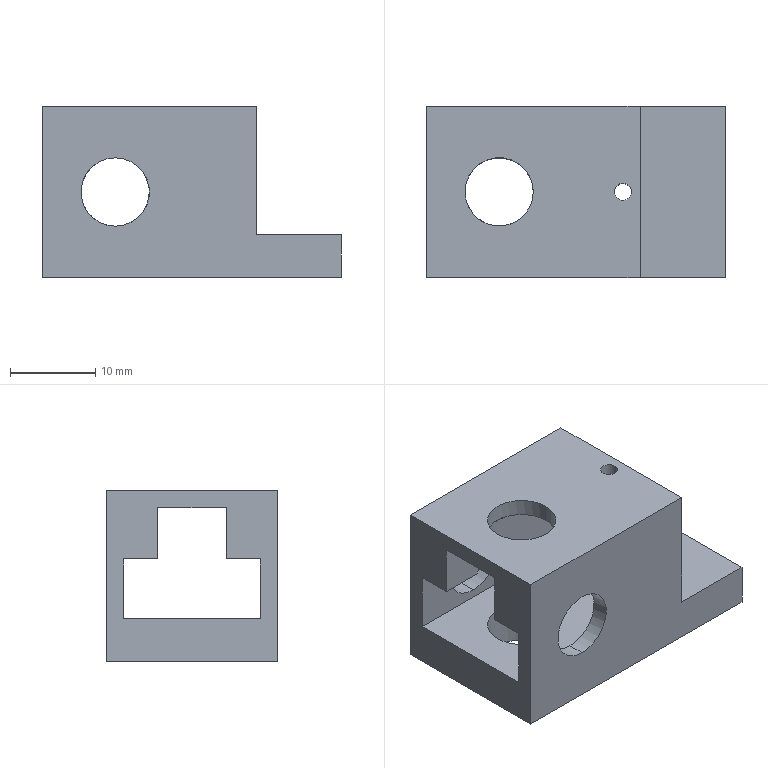Part | SolidWorks | features ICE 3, Extrusion 1 | 1 solid | 30 faces | box 35 x 20 x 20 mm | volume 6348 mm3 | plane 18 | cylinder 12 | commonest cylinder face diameters 8 x8 2 x4
STEP:
#1=CARTESIAN_POINT('',(8.5,0.,-14.));
#2=VERTEX_POINT('',#1);
#3=CARTESIAN_POINT('',(8.5,0.,-6.));
#4=VERTEX_POINT('',#3);
#5=CARTESIAN_POINT('',(8.5,0.,-10.));
#6=DIRECTION('',(0.,1.,0.));
#7=DIRECTION('',(0.,0.,1.));
#8=AXIS2_PLACEMENT_3D('',#5,#6,#7);
#9=CIRCLE('',#8,4.);
#10=EDGE_CURVE('',#2,#4,#9,.T.);
#11=ORIENTED_EDGE('',*,*,#10,.F.);
#12=CARTESIAN_POINT('',(8.5,2.005,-14.));
#13=VERTEX_POINT('',#12);
#14=CARTESIAN_POINT('',(8.5,0.,-14.));
#15=DIRECTION('',(0.,1.,0.));
#16=VECTOR('',#15,1000.);
#17=LINE('',#14,#16);
#18=EDGE_CURVE('',#2,#13,#17,.T.);
#19=ORIENTED_EDGE('',*,*,#18,.T.);
#20=CARTESIAN_POINT('',(5.036,2.005,-8.));
#21=VERTEX_POINT('',#20);
#22=CARTESIAN_POINT('',(8.5,2.005,-10.));
#23=DIRECTION('',(0.,1.,0.));
#24=DIRECTION('',(0.,0.,-1.));
#25=AXIS2_PLACEMENT_3D('',#22,#23,#24);
#26=CIRCLE('',#25,4.);
#27=EDGE_CURVE('',#13,#21,#26,.T.);
#28=ORIENTED_EDGE('',*,*,#27,.T.);
#29=CARTESIAN_POINT('',(5.036,6.,-8.));
#30=VERTEX_POINT('',#29);
#31=CARTESIAN_POINT('',(5.036,0.,-8.));
#32=DIRECTION('',(0.,1.,0.));
#33=VECTOR('',#32,1000.);
#34=LINE('',#31,#33);
#35=EDGE_CURVE('',#21,#30,#34,.T.);
#36=ORIENTED_EDGE('',*,*,#35,.T.);
#37=CARTESIAN_POINT('',(8.5,6.,-6.));
#38=VERTEX_POINT('',#37);
#39=CARTESIAN_POINT('',(8.5,6.,-10.));
#40=DIRECTION('',(0.,1.,0.));
#41=DIRECTION('',(0.,0.,-1.));
#42=AXIS2_PLACEMENT_3D('',#39,#40,#41);
#43=CIRCLE('',#42,4.);
#44=EDGE_CURVE('',#30,#38,#43,.T.);
#45=ORIENTED_EDGE('',*,*,#44,.T.);
#46=CARTESIAN_POINT('',(8.5,0.,-6.));
#47=DIRECTION('',(0.,1.,0.));
#48=VECTOR('',#47,1000.);
#49=LINE('',#46,#48);
#50=EDGE_CURVE('',#4,#38,#49,.T.);
#51=ORIENTED_EDGE('',*,*,#50,.F.);
#52=EDGE_LOOP('',(#11,#19,#28,#36,#45,#51));
#53=FACE_OUTER_BOUND('',#52,.T.);
#54=CARTESIAN_POINT('',(8.5,0.,-10.));
#55=DIRECTION('',(0.,1.,0.));
#56=DIRECTION('',(0.,0.,1.));
#57=AXIS2_PLACEMENT_3D('',#54,#55,#56);
#58=CYLINDRICAL_SURFACE('',#57,4.);
#59=ADVANCED_FACE('',(#53),#58,.F.);
#60=CARTESIAN_POINT('',(5.036,17.995,-8.));
#61=VERTEX_POINT('',#60);
#62=CARTESIAN_POINT('',(8.5,17.995,-14.));
#63=VERTEX_POINT('',#62);
#64=CARTESIAN_POINT('',(8.5,17.995,-10.));
#65=DIRECTION('',(0.,-1.,0.));
#66=DIRECTION('',(0.,0.,1.));
#67=AXIS2_PLACEMENT_3D('',#64,#65,#66);
#68=CIRCLE('',#67,4.);
#69=EDGE_CURVE('',#61,#63,#68,.T.);
#70=ORIENTED_EDGE('',*,*,#69,.T.);
#71=CARTESIAN_POINT('',(8.5,20.,-14.));
#72=VERTEX_POINT('',#71);
#73=CARTESIAN_POINT('',(8.5,0.,-14.));
#74=DIRECTION('',(0.,1.,0.));
#75=VECTOR('',#74,1000.);
#76=LINE('',#73,#75);
#77=EDGE_CURVE('',#63,#72,#76,.T.);
#78=ORIENTED_EDGE('',*,*,#77,.T.);
#79=CARTESIAN_POINT('',(8.5,20.,-6.));
#80=VERTEX_POINT('',#79);
#81=CARTESIAN_POINT('',(8.5,20.,-10.));
#82=DIRECTION('',(0.,1.,0.));
#83=DIRECTION('',(0.,0.,1.));
#84=AXIS2_PLACEMENT_3D('',#81,#82,#83);
#85=CIRCLE('',#84,4.);
#86=EDGE_CURVE('',#72,#80,#85,.T.);
#87=ORIENTED_EDGE('',*,*,#86,.T.);
#88=CARTESIAN_POINT('',(8.5,14.,-6.));
#89=VERTEX_POINT('',#88);
#90=CARTESIAN_POINT('',(8.5,0.,-6.));
#91=DIRECTION('',(0.,1.,0.));
#92=VECTOR('',#91,1000.);
#93=LINE('',#90,#92);
#94=EDGE_CURVE('',#89,#80,#93,.T.);
#95=ORIENTED_EDGE('',*,*,#94,.F.);
#96=CARTESIAN_POINT('',(5.036,14.,-8.));
#97=VERTEX_POINT('',#96);
#98=CARTESIAN_POINT('',(8.5,14.,-10.));
#99=DIRECTION('',(0.,-1.,0.));
#100=DIRECTION('',(0.,0.,1.));
#101=AXIS2_PLACEMENT_3D('',#98,#99,#100);
#102=CIRCLE('',#101,4.);
#103=EDGE_CURVE('',#89,#97,#102,.T.);
#104=ORIENTED_EDGE('',*,*,#103,.T.);
#105=CARTESIAN_POINT('',(5.036,0.,-8.));
#106=DIRECTION('',(0.,1.,0.));
#107=VECTOR('',#106,1000.);
#108=LINE('',#105,#107);
#109=EDGE_CURVE('',#97,#61,#108,.T.);
#110=ORIENTED_EDGE('',*,*,#109,.T.);
#111=EDGE_LOOP('',(#70,#78,#87,#95,#104,#110));
#112=FACE_OUTER_BOUND('',#111,.T.);
#113=CARTESIAN_POINT('',(8.5,0.,-10.));
#114=DIRECTION('',(0.,1.,0.));
#115=DIRECTION('',(0.,0.,1.));
#116=AXIS2_PLACEMENT_3D('',#113,#114,#115);
#117=CYLINDRICAL_SURFACE('',#116,4.);
#118=ADVANCED_FACE('',(#112),#117,.F.);
#119=CARTESIAN_POINT('',(4.5,10.,-20.));
#120=VERTEX_POINT('',#119);
#121=CARTESIAN_POINT('',(12.5,10.,-20.));
#122=VERTEX_POINT('',#121);
#123=CARTESIAN_POINT('',(8.5,10.,-20.));
#124=DIRECTION('',(0.,0.,1.));
#125=DIRECTION('',(1.,0.,0.));
#126=AXIS2_PLACEMENT_3D('',#123,#124,#125);
#127=CIRCLE('',#126,4.);
#128=EDGE_CURVE('',#120,#122,#127,.T.);
#129=ORIENTED_EDGE('',*,*,#128,.F.);
#130=CARTESIAN_POINT('',(4.5,10.,-15.));
#131=VERTEX_POINT('',#130);
#132=CARTESIAN_POINT('',(4.5,10.,-20.));
#133=DIRECTION('',(0.,0.,1.));
#134=VECTOR('',#133,1000.);
#135=LINE('',#132,#134);
#136=EDGE_CURVE('',#120,#131,#135,.T.);
#137=ORIENTED_EDGE('',*,*,#136,.T.);
#138=CARTESIAN_POINT('',(12.5,10.,-15.));
#139=VERTEX_POINT('',#138);
#140=CARTESIAN_POINT('',(8.5,10.,-15.));
#141=DIRECTION('',(0.,0.,1.));
#142=DIRECTION('',(-1.,0.,0.));
#143=AXIS2_PLACEMENT_3D('',#140,#141,#142);
#144=CIRCLE('',#143,4.);
#145=EDGE_CURVE('',#131,#139,#144,.T.);
#146=ORIENTED_EDGE('',*,*,#145,.T.);
#147=CARTESIAN_POINT('',(12.5,10.,-20.));
#148=DIRECTION('',(0.,0.,1.));
#149=VECTOR('',#148,1000.);
#150=LINE('',#147,#149);
#151=EDGE_CURVE('',#122,#139,#150,.T.);
#152=ORIENTED_EDGE('',*,*,#151,.F.);
#153=EDGE_LOOP('',(#129,#137,#146,#152));
#154=FACE_OUTER_BOUND('',#153,.T.);
#155=CARTESIAN_POINT('',(8.5,10.,-20.));
#156=DIRECTION('',(0.,0.,1.));
#157=DIRECTION('',(1.,0.,0.));
#158=AXIS2_PLACEMENT_3D('',#155,#156,#157);
#159=CYLINDRICAL_SURFACE('',#158,4.);
#160=ADVANCED_FACE('',(#154),#159,.F.);
#161=CARTESIAN_POINT('',(24.,10.,-2.));
#162=VERTEX_POINT('',#161);
#163=CARTESIAN_POINT('',(22.,10.,-2.));
#164=VERTEX_POINT('',#163);
#165=CARTESIAN_POINT('',(23.,10.,-2.));
#166=DIRECTION('',(0.,0.,-1.));
#167=DIRECTION('',(0.,-1.,0.));
#168=AXIS2_PLACEMENT_3D('',#165,#166,#167);
#169=CIRCLE('',#168,1.);
#170=EDGE_CURVE('',#162,#164,#169,.T.);
#171=ORIENTED_EDGE('',*,*,#170,.T.);
#172=CARTESIAN_POINT('',(22.,10.,0.));
#173=VERTEX_POINT('',#172);
#174=CARTESIAN_POINT('',(22.,10.,-20.));
#175=DIRECTION('',(0.,0.,1.));
#176=VECTOR('',#175,1000.);
#177=LINE('',#174,#176);
#178=EDGE_CURVE('',#164,#173,#177,.T.);
#179=ORIENTED_EDGE('',*,*,#178,.T.);
#180=CARTESIAN_POINT('',(24.,10.,0.));
#181=VERTEX_POINT('',#180);
#182=CARTESIAN_POINT('',(23.,10.,0.));
#183=DIRECTION('',(0.,0.,-1.));
#184=DIRECTION('',(-1.,0.,0.));
#185=AXIS2_PLACEMENT_3D('',#182,#183,#184);
#186=CIRCLE('',#185,1.);
#187=EDGE_CURVE('',#181,#173,#186,.T.);
#188=ORIENTED_EDGE('',*,*,#187,.F.);
#189=CARTESIAN_POINT('',(24.,10.,-20.));
#190=DIRECTION('',(0.,0.,1.));
#191=VECTOR('',#190,1000.);
#192=LINE('',#189,#191);
#193=EDGE_CURVE('',#162,#181,#192,.T.);
#194=ORIENTED_EDGE('',*,*,#193,.F.);
#195=EDGE_LOOP('',(#171,#179,#188,#194));
#196=FACE_OUTER_BOUND('',#195,.T.);
#197=CARTESIAN_POINT('',(23.,10.,-20.));
#198=DIRECTION('',(0.,0.,1.));
#199=DIRECTION('',(1.,0.,0.));
#200=AXIS2_PLACEMENT_3D('',#197,#198,#199);
#201=CYLINDRICAL_SURFACE('',#200,1.);
#202=ADVANCED_FACE('',(#196),#201,.F.);
#203=CARTESIAN_POINT('',(8.5,6.,-2.));
#204=VERTEX_POINT('',#203);
#205=CARTESIAN_POINT('',(4.5,10.,-2.));
#206=VERTEX_POINT('',#205);
#207=CARTESIAN_POINT('',(8.5,10.,-2.));
#208=DIRECTION('',(0.,0.,-1.));
#209=DIRECTION('',(0.,-1.,0.));
#210=AXIS2_PLACEMENT_3D('',#207,#208,#209);
#211=CIRCLE('',#210,4.);
#212=EDGE_CURVE('',#204,#206,#211,.T.);
#213=ORIENTED_EDGE('',*,*,#212,.T.);
#214=CARTESIAN_POINT('',(4.5,10.,0.));
#215=VERTEX_POINT('',#214);
#216=CARTESIAN_POINT('',(4.5,10.,-20.));
#217=DIRECTION('',(0.,0.,1.));
#218=VECTOR('',#217,1000.);
#219=LINE('',#216,#218);
#220=EDGE_CURVE('',#206,#215,#219,.T.);
#221=ORIENTED_EDGE('',*,*,#220,.T.);
#222=CARTESIAN_POINT('',(12.5,10.,0.));
#223=VERTEX_POINT('',#222);
#224=CARTESIAN_POINT('',(8.5,10.,0.));
#225=DIRECTION('',(0.,0.,-1.));
#226=DIRECTION('',(-1.,0.,0.));
#227=AXIS2_PLACEMENT_3D('',#224,#225,#226);
#228=CIRCLE('',#227,4.);
#229=EDGE_CURVE('',#223,#215,#228,.T.);
#230=ORIENTED_EDGE('',*,*,#229,.F.);
#231=CARTESIAN_POINT('',(12.5,10.,-2.));
#232=VERTEX_POINT('',#231);
#233=CARTESIAN_POINT('',(12.5,10.,-20.));
#234=DIRECTION('',(0.,0.,1.));
#235=VECTOR('',#234,1000.);
#236=LINE('',#233,#235);
#237=EDGE_CURVE('',#232,#223,#236,.T.);
#238=ORIENTED_EDGE('',*,*,#237,.F.);
#239=CARTESIAN_POINT('',(8.5,10.,-2.));
#240=DIRECTION('',(0.,0.,-1.));
#241=DIRECTION('',(0.,-1.,0.));
#242=AXIS2_PLACEMENT_3D('',#239,#240,#241);
#243=CIRCLE('',#242,4.);
#244=EDGE_CURVE('',#232,#204,#243,.T.);
#245=ORIENTED_EDGE('',*,*,#244,.T.);
#246=EDGE_LOOP('',(#213,#221,#230,#238,#245));
#247=FACE_OUTER_BOUND('',#246,.T.);
#248=CARTESIAN_POINT('',(8.5,10.,-20.));
#249=DIRECTION('',(0.,0.,1.));
#250=DIRECTION('',(1.,0.,0.));
#251=AXIS2_PLACEMENT_3D('',#248,#249,#250);
#252=CYLINDRICAL_SURFACE('',#251,4.);
#253=ADVANCED_FACE('',(#247),#252,.F.);
#254=CARTESIAN_POINT('',(22.,10.,-20.));
#255=VERTEX_POINT('',#254);
#256=CARTESIAN_POINT('',(24.,10.,-20.));
#257=VERTEX_POINT('',#256);
#258=CARTESIAN_POINT('',(23.,10.,-20.));
#259=DIRECTION('',(0.,0.,1.));
#260=DIRECTION('',(1.,0.,0.));
#261=AXIS2_PLACEMENT_3D('',#258,#259,#260);
#262=CIRCLE('',#261,1.);
#263=EDGE_CURVE('',#255,#257,#262,.T.);
#264=ORIENTED_EDGE('',*,*,#263,.F.);
#265=CARTESIAN_POINT('',(22.,10.,-15.));
#266=VERTEX_POINT('',#265);
#267=CARTESIAN_POINT('',(22.,10.,-20.));
#268=DIRECTION('',(0.,0.,1.));
#269=VECTOR('',#268,1000.);
#270=LINE('',#267,#269);
#271=EDGE_CURVE('',#255,#266,#270,.T.);
#272=ORIENTED_EDGE('',*,*,#271,.T.);
#273=CARTESIAN_POINT('',(24.,10.,-15.));
#274=VERTEX_POINT('',#273);
#275=CARTESIAN_POINT('',(23.,10.,-15.));
#276=DIRECTION('',(0.,0.,1.));
#277=DIRECTION('',(-1.,0.,0.));
#278=AXIS2_PLACEMENT_3D('',#275,#276,#277);
#279=CIRCLE('',#278,1.);
#280=EDGE_CURVE('',#266,#274,#279,.T.);
#281=ORIENTED_EDGE('',*,*,#280,.T.);
#282=CARTESIAN_POINT('',(24.,10.,-20.));
#283=DIRECTION('',(0.,0.,1.));
#284=VECTOR('',#283,1000.);
#285=LINE('',#282,#284);
#286=EDGE_CURVE('',#257,#274,#285,.T.);
#287=ORIENTED_EDGE('',*,*,#286,.F.);
#288=EDGE_LOOP('',(#264,#272,#281,#287));
#289=FACE_OUTER_BOUND('',#288,.T.);
#290=CARTESIAN_POINT('',(23.,10.,-20.));
#291=DIRECTION('',(0.,0.,1.));
#292=DIRECTION('',(1.,0.,0.));
#293=AXIS2_PLACEMENT_3D('',#290,#291,#292);
#294=CYLINDRICAL_SURFACE('',#293,1.);
#295=ADVANCED_FACE('',(#289),#294,.F.);
#296=ORIENTED_EDGE('',*,*,#271,.F.);
#297=CARTESIAN_POINT('',(23.,10.,-20.));
#298=DIRECTION('',(0.,0.,1.));
#299=DIRECTION('',(1.,0.,0.));
#300=AXIS2_PLACEMENT_3D('',#297,#298,#299);
#301=CIRCLE('',#300,1.);
#302=EDGE_CURVE('',#257,#255,#301,.T.);
#303=ORIENTED_EDGE('',*,*,#302,.F.);
#304=ORIENTED_EDGE('',*,*,#286,.T.);
#305=CARTESIAN_POINT('',(23.,10.,-15.));
#306=DIRECTION('',(0.,0.,1.));
#307=DIRECTION('',(-1.,0.,0.));
#308=AXIS2_PLACEMENT_3D('',#305,#306,#307);
#309=CIRCLE('',#308,1.);
#310=EDGE_CURVE('',#274,#266,#309,.T.);
#311=ORIENTED_EDGE('',*,*,#310,.T.);
#312=EDGE_LOOP('',(#296,#303,#304,#311));
#313=FACE_OUTER_BOUND('',#312,.T.);
#314=CARTESIAN_POINT('',(23.,10.,-20.));
#315=DIRECTION('',(0.,0.,1.));
#316=DIRECTION('',(1.,0.,0.));
#317=AXIS2_PLACEMENT_3D('',#314,#315,#316);
#318=CYLINDRICAL_SURFACE('',#317,1.);
#319=ADVANCED_FACE('',(#313),#318,.F.);
#320=ORIENTED_EDGE('',*,*,#220,.F.);
#321=CARTESIAN_POINT('',(8.5,14.,-2.));
#322=VERTEX_POINT('',#321);
#323=CARTESIAN_POINT('',(8.5,10.,-2.));
#324=DIRECTION('',(0.,0.,-1.));
#325=DIRECTION('',(0.,-1.,0.));
#326=AXIS2_PLACEMENT_3D('',#323,#324,#325);
#327=CIRCLE('',#326,4.);
#328=EDGE_CURVE('',#206,#322,#327,.T.);
#329=ORIENTED_EDGE('',*,*,#328,.T.);
#330=CARTESIAN_POINT('',(8.5,10.,-2.));
#331=DIRECTION('',(0.,0.,-1.));
#332=DIRECTION('',(0.,-1.,0.));
#333=AXIS2_PLACEMENT_3D('',#330,#331,#332);
#334=CIRCLE('',#333,4.);
#335=EDGE_CURVE('',#322,#232,#334,.T.);
#336=ORIENTED_EDGE('',*,*,#335,.T.);
#337=ORIENTED_EDGE('',*,*,#237,.T.);
#338=CARTESIAN_POINT('',(8.5,10.,0.));
#339=DIRECTION('',(0.,0.,-1.));
#340=DIRECTION('',(-1.,0.,0.));
#341=AXIS2_PLACEMENT_3D('',#338,#339,#340);
#342=CIRCLE('',#341,4.);
#343=EDGE_CURVE('',#215,#223,#342,.T.);
#344=ORIENTED_EDGE('',*,*,#343,.F.);
#345=EDGE_LOOP('',(#320,#329,#336,#337,#344));
#346=FACE_OUTER_BOUND('',#345,.T.);
#347=CARTESIAN_POINT('',(8.5,10.,-20.));
#348=DIRECTION('',(0.,0.,1.));
#349=DIRECTION('',(1.,0.,0.));
#350=AXIS2_PLACEMENT_3D('',#347,#348,#349);
#351=CYLINDRICAL_SURFACE('',#350,4.);
#352=ADVANCED_FACE('',(#346),#351,.F.);
#353=CARTESIAN_POINT('',(0.,2.005,-15.));
#354=VERTEX_POINT('',#353);
#355=CARTESIAN_POINT('',(0.,17.995,-15.));
#356=VERTEX_POINT('',#355);
#357=CARTESIAN_POINT('',(0.,2.005,-15.));
#358=DIRECTION('',(0.,1.,0.));
#359=VECTOR('',#358,1000.);
#360=LINE('',#357,#359);
#361=EDGE_CURVE('',#354,#356,#360,.T.);
#362=ORIENTED_EDGE('',*,*,#361,.T.);
#363=CARTESIAN_POINT('',(0.,17.995,-8.));
#364=VERTEX_POINT('',#363);
#365=CARTESIAN_POINT('',(0.,17.995,-8.));
#366=DIRECTION('',(0.,0.,1.));
#367=VECTOR('',#366,1000.);
#368=LINE('',#365,#367);
#369=EDGE_CURVE('',#356,#364,#368,.T.);
#370=ORIENTED_EDGE('',*,*,#369,.T.);
#371=CARTESIAN_POINT('',(0.,14.,-8.));
#372=VERTEX_POINT('',#371);
#373=CARTESIAN_POINT('',(0.,14.,-8.));
#374=DIRECTION('',(0.,-1.,0.));
#375=VECTOR('',#374,1000.);
#376=LINE('',#373,#375);
#377=EDGE_CURVE('',#364,#372,#376,.T.);
#378=ORIENTED_EDGE('',*,*,#377,.T.);
#379=CARTESIAN_POINT('',(0.,14.,-2.));
#380=VERTEX_POINT('',#379);
#381=CARTESIAN_POINT('',(0.,14.,-2.));
#382=DIRECTION('',(0.,0.,1.));
#383=VECTOR('',#382,1000.);
#384=LINE('',#381,#383);
#385=EDGE_CURVE('',#372,#380,#384,.T.);
#386=ORIENTED_EDGE('',*,*,#385,.T.);
#387=CARTESIAN_POINT('',(0.,6.,-2.));
#388=VERTEX_POINT('',#387);
#389=CARTESIAN_POINT('',(0.,14.,-2.));
#390=DIRECTION('',(0.,-1.,0.));
#391=VECTOR('',#390,1000.);
#392=LINE('',#389,#391);
#393=EDGE_CURVE('',#380,#388,#392,.T.);
#394=ORIENTED_EDGE('',*,*,#393,.T.);
#395=CARTESIAN_POINT('',(0.,6.,-8.));
#396=VERTEX_POINT('',#395);
#397=CARTESIAN_POINT('',(0.,6.,-2.));
#398=DIRECTION('',(0.,0.,-1.));
#399=VECTOR('',#398,1000.);
#400=LINE('',#397,#399);
#401=EDGE_CURVE('',#388,#396,#400,.T.);
#402=ORIENTED_EDGE('',*,*,#401,.T.);
#403=CARTESIAN_POINT('',(0.,2.005,-8.));
#404=VERTEX_POINT('',#403);
#405=CARTESIAN_POINT('',(0.,6.,-8.));
#406=DIRECTION('',(0.,-1.,0.));
#407=VECTOR('',#406,1000.);
#408=LINE('',#405,#407);
#409=EDGE_CURVE('',#396,#404,#408,.T.);
#410=ORIENTED_EDGE('',*,*,#409,.T.);
#411=CARTESIAN_POINT('',(0.,2.005,-8.));
#412=DIRECTION('',(0.,0.,-1.));
#413=VECTOR('',#412,1000.);
#414=LINE('',#411,#413);
#415=EDGE_CURVE('',#404,#354,#414,.T.);
#416=ORIENTED_EDGE('',*,*,#415,.T.);
#417=EDGE_LOOP('',(#362,#370,#378,#386,#394,#402,#410,#416));
#418=FACE_BOUND('',#417,.T.);
#419=CARTESIAN_POINT('',(0.,0.,-20.));
#420=VERTEX_POINT('',#419);
#421=CARTESIAN_POINT('',(0.,0.,0.));
#422=VERTEX_POINT('',#421);
#423=CARTESIAN_POINT('',(0.,0.,-20.));
#424=DIRECTION('',(0.,0.,1.));
#425=VECTOR('',#424,1000.);
#426=LINE('',#423,#425);
#427=EDGE_CURVE('',#420,#422,#426,.T.);
#428=ORIENTED_EDGE('',*,*,#427,.T.);
#429=CARTESIAN_POINT('',(0.,20.,0.));
#430=VERTEX_POINT('',#429);
#431=CARTESIAN_POINT('',(0.,20.,0.));
#432=DIRECTION('',(0.,-1.,0.));
#433=VECTOR('',#432,1000.);
#434=LINE('',#431,#433);
#435=EDGE_CURVE('',#430,#422,#434,.T.);
#436=ORIENTED_EDGE('',*,*,#435,.F.);
#437=CARTESIAN_POINT('',(0.,20.,-20.));
#438=VERTEX_POINT('',#437);
#439=CARTESIAN_POINT('',(0.,20.,-20.));
#440=DIRECTION('',(0.,0.,1.));
#441=VECTOR('',#440,1000.);
#442=LINE('',#439,#441);
#443=EDGE_CURVE('',#438,#430,#442,.T.);
#444=ORIENTED_EDGE('',*,*,#443,.F.);
#445=CARTESIAN_POINT('',(0.,20.,-20.));
#446=DIRECTION('',(0.,-1.,0.));
#447=VECTOR('',#446,1000.);
#448=LINE('',#445,#447);
#449=EDGE_CURVE('',#438,#420,#448,.T.);
#450=ORIENTED_EDGE('',*,*,#449,.T.);
#451=EDGE_LOOP('',(#428,#436,#444,#450));
#452=FACE_OUTER_BOUND('',#451,.T.);
#453=CARTESIAN_POINT('',(0.,20.,-20.));
#454=DIRECTION('',(1.,0.,0.));
#455=DIRECTION('',(0.,0.,-1.));
#456=AXIS2_PLACEMENT_3D('',#453,#454,#455);
#457=PLANE('',#456);
#458=ADVANCED_FACE('',(#418,#452),#457,.F.);
#459=ORIENTED_EDGE('',*,*,#229,.T.);
#460=ORIENTED_EDGE('',*,*,#343,.T.);
#461=EDGE_LOOP('',(#459,#460));
#462=FACE_BOUND('',#461,.T.);
#463=ORIENTED_EDGE('',*,*,#187,.T.);
#464=CARTESIAN_POINT('',(23.,10.,0.));
#465=DIRECTION('',(0.,0.,-1.));
#466=DIRECTION('',(-1.,0.,0.));
#467=AXIS2_PLACEMENT_3D('',#464,#465,#466);
#468=CIRCLE('',#467,1.);
#469=EDGE_CURVE('',#173,#181,#468,.T.);
#470=ORIENTED_EDGE('',*,*,#469,.T.);
#471=EDGE_LOOP('',(#463,#470));
#472=FACE_BOUND('',#471,.T.);
#473=CARTESIAN_POINT('',(25.,0.,0.));
#474=VERTEX_POINT('',#473);
#475=CARTESIAN_POINT('',(0.,0.,0.));
#476=DIRECTION('',(1.,0.,0.));
#477=VECTOR('',#476,1000.);
#478=LINE('',#475,#477);
#479=EDGE_CURVE('',#422,#474,#478,.T.);
#480=ORIENTED_EDGE('',*,*,#479,.T.);
#481=CARTESIAN_POINT('',(25.,20.,0.));
#482=VERTEX_POINT('',#481);
#483=CARTESIAN_POINT('',(25.,20.,0.));
#484=DIRECTION('',(0.,-1.,0.));
#485=VECTOR('',#484,1000.);
#486=LINE('',#483,#485);
#487=EDGE_CURVE('',#482,#474,#486,.T.);
#488=ORIENTED_EDGE('',*,*,#487,.F.);
#489=CARTESIAN_POINT('',(0.,20.,0.));
#490=DIRECTION('',(1.,0.,0.));
#491=VECTOR('',#490,1000.);
#492=LINE('',#489,#491);
#493=EDGE_CURVE('',#430,#482,#492,.T.);
#494=ORIENTED_EDGE('',*,*,#493,.F.);
#495=ORIENTED_EDGE('',*,*,#435,.T.);
#496=EDGE_LOOP('',(#480,#488,#494,#495));
#497=FACE_OUTER_BOUND('',#496,.T.);
#498=CARTESIAN_POINT('',(0.,20.,0.));
#499=DIRECTION('',(0.,0.,-1.));
#500=DIRECTION('',(-1.,0.,0.));
#501=AXIS2_PLACEMENT_3D('',#498,#499,#500);
#502=PLANE('',#501);
#503=ADVANCED_FACE('',(#462,#472,#497),#502,.F.);
#504=CARTESIAN_POINT('',(25.,17.995,-8.));
#505=VERTEX_POINT('',#504);
#506=CARTESIAN_POINT('',(25.,14.,-8.));
#507=VERTEX_POINT('',#506);
#508=CARTESIAN_POINT('',(25.,14.,-8.));
#509=DIRECTION('',(0.,-1.,0.));
#510=VECTOR('',#509,1000.);
#511=LINE('',#508,#510);
#512=EDGE_CURVE('',#505,#507,#511,.T.);
#513=ORIENTED_EDGE('',*,*,#512,.F.);
#514=CARTESIAN_POINT('',(25.,17.995,-15.));
#515=VERTEX_POINT('',#514);
#516=CARTESIAN_POINT('',(25.,17.995,-8.));
#517=DIRECTION('',(0.,0.,1.));
#518=VECTOR('',#517,1000.);
#519=LINE('',#516,#518);
#520=EDGE_CURVE('',#515,#505,#519,.T.);
#521=ORIENTED_EDGE('',*,*,#520,.F.);
#522=CARTESIAN_POINT('',(25.,20.,-15.));
#523=VERTEX_POINT('',#522);
#524=CARTESIAN_POINT('',(25.,20.,-15.));
#525=DIRECTION('',(0.,-1.,0.));
#526=VECTOR('',#525,1000.);
#527=LINE('',#524,#526);
#528=EDGE_CURVE('',#523,#515,#527,.T.);
#529=ORIENTED_EDGE('',*,*,#528,.F.);
#530=CARTESIAN_POINT('',(25.,20.,0.));
#531=DIRECTION('',(0.,0.,-1.));
#532=VECTOR('',#531,1000.);
#533=LINE('',#530,#532);
#534=EDGE_CURVE('',#482,#523,#533,.T.);
#535=ORIENTED_EDGE('',*,*,#534,.F.);
#536=ORIENTED_EDGE('',*,*,#487,.T.);
#537=CARTESIAN_POINT('',(25.,0.,-15.));
#538=VERTEX_POINT('',#537);
#539=CARTESIAN_POINT('',(25.,0.,0.));
#540=DIRECTION('',(0.,0.,-1.));
#541=VECTOR('',#540,1000.);
#542=LINE('',#539,#541);
#543=EDGE_CURVE('',#474,#538,#542,.T.);
#544=ORIENTED_EDGE('',*,*,#543,.T.);
#545=CARTESIAN_POINT('',(25.,2.005,-15.));
#546=VERTEX_POINT('',#545);
#547=CARTESIAN_POINT('',(25.,20.,-15.));
#548=DIRECTION('',(0.,-1.,0.));
#549=VECTOR('',#548,1000.);
#550=LINE('',#547,#549);
#551=EDGE_CURVE('',#546,#538,#550,.T.);
#552=ORIENTED_EDGE('',*,*,#551,.F.);
#553=CARTESIAN_POINT('',(25.,2.005,-8.));
#554=VERTEX_POINT('',#553);
#555=CARTESIAN_POINT('',(25.,2.005,-8.));
#556=DIRECTION('',(0.,0.,-1.));
#557=VECTOR('',#556,1000.);
#558=LINE('',#555,#557);
#559=EDGE_CURVE('',#554,#546,#558,.T.);
#560=ORIENTED_EDGE('',*,*,#559,.F.);
#561=CARTESIAN_POINT('',(25.,6.,-8.));
#562=VERTEX_POINT('',#561);
#563=CARTESIAN_POINT('',(25.,6.,-8.));
#564=DIRECTION('',(0.,-1.,0.));
#565=VECTOR('',#564,1000.);
#566=LINE('',#563,#565);
#567=EDGE_CURVE('',#562,#554,#566,.T.);
#568=ORIENTED_EDGE('',*,*,#567,.F.);
#569=CARTESIAN_POINT('',(25.,6.,-2.));
#570=VERTEX_POINT('',#569);
#571=CARTESIAN_POINT('',(25.,6.,-2.));
#572=DIRECTION('',(0.,0.,-1.));
#573=VECTOR('',#572,1000.);
#574=LINE('',#571,#573);
#575=EDGE_CURVE('',#570,#562,#574,.T.);
#576=ORIENTED_EDGE('',*,*,#575,.F.);
#577=CARTESIAN_POINT('',(25.,14.,-2.));
#578=VERTEX_POINT('',#577);
#579=CARTESIAN_POINT('',(25.,14.,-2.));
#580=DIRECTION('',(0.,-1.,0.));
#581=VECTOR('',#580,1000.);
#582=LINE('',#579,#581);
#583=EDGE_CURVE('',#578,#570,#582,.T.);
#584=ORIENTED_EDGE('',*,*,#583,.F.);
#585=CARTESIAN_POINT('',(25.,14.,-2.));
#586=DIRECTION('',(0.,0.,1.));
#587=VECTOR('',#586,1000.);
#588=LINE('',#585,#587);
#589=EDGE_CURVE('',#507,#578,#588,.T.);
#590=ORIENTED_EDGE('',*,*,#589,.F.);
#591=EDGE_LOOP('',(#513,#521,#529,#535,#536,#544,#552,#560,#568,#576,#584,#590));
#592=FACE_OUTER_BOUND('',#591,.T.);
#593=CARTESIAN_POINT('',(25.,20.,0.));
#594=DIRECTION('',(-1.,0.,0.));
#595=DIRECTION('',(0.,0.,1.));
#596=AXIS2_PLACEMENT_3D('',#593,#594,#595);
#597=PLANE('',#596);
#598=ADVANCED_FACE('',(#592),#597,.F.);
#599=CARTESIAN_POINT('',(35.,0.,-15.));
#600=VERTEX_POINT('',#599);
#601=CARTESIAN_POINT('',(25.,0.,-15.));
#602=DIRECTION('',(1.,0.,0.));
#603=VECTOR('',#602,1000.);
#604=LINE('',#601,#603);
#605=EDGE_CURVE('',#538,#600,#604,.T.);
#606=ORIENTED_EDGE('',*,*,#605,.T.);
#607=CARTESIAN_POINT('',(35.,20.,-15.));
#608=VERTEX_POINT('',#607);
#609=CARTESIAN_POINT('',(35.,20.,-15.));
#610=DIRECTION('',(0.,-1.,0.));
#611=VECTOR('',#610,1000.);
#612=LINE('',#609,#611);
#613=EDGE_CURVE('',#608,#600,#612,.T.);
#614=ORIENTED_EDGE('',*,*,#613,.F.);
#615=CARTESIAN_POINT('',(25.,20.,-15.));
#616=DIRECTION('',(1.,0.,0.));
#617=VECTOR('',#616,1000.);
#618=LINE('',#615,#617);
#619=EDGE_CURVE('',#523,#608,#618,.T.);
#620=ORIENTED_EDGE('',*,*,#619,.F.);
#621=ORIENTED_EDGE('',*,*,#528,.T.);
#622=CARTESIAN_POINT('',(0.,17.995,-15.));
#623=DIRECTION('',(1.,0.,0.));
#624=VECTOR('',#623,1000.);
#625=LINE('',#622,#624);
#626=EDGE_CURVE('',#356,#515,#625,.T.);
#627=ORIENTED_EDGE('',*,*,#626,.F.);
#628=ORIENTED_EDGE('',*,*,#361,.F.);
#629=CARTESIAN_POINT('',(0.,2.005,-15.));
#630=DIRECTION('',(1.,0.,0.));
#631=VECTOR('',#630,1000.);
#632=LINE('',#629,#631);
#633=EDGE_CURVE('',#354,#546,#632,.T.);
#634=ORIENTED_EDGE('',*,*,#633,.T.);
#635=ORIENTED_EDGE('',*,*,#551,.T.);
#636=EDGE_LOOP('',(#606,#614,#620,#621,#627,#628,#634,#635));
#637=FACE_OUTER_BOUND('',#636,.T.);
#638=CARTESIAN_POINT('',(8.5,10.,-15.));
#639=DIRECTION('',(0.,0.,1.));
#640=DIRECTION('',(-1.,0.,0.));
#641=AXIS2_PLACEMENT_3D('',#638,#639,#640);
#642=CIRCLE('',#641,4.);
#643=EDGE_CURVE('',#139,#131,#642,.T.);
#644=ORIENTED_EDGE('',*,*,#643,.F.);
#645=ORIENTED_EDGE('',*,*,#145,.F.);
#646=EDGE_LOOP('',(#644,#645));
#647=FACE_BOUND('',#646,.T.);
#648=ORIENTED_EDGE('',*,*,#310,.F.);
#649=ORIENTED_EDGE('',*,*,#280,.F.);
#650=EDGE_LOOP('',(#648,#649));
#651=FACE_BOUND('',#650,.T.);
#652=CARTESIAN_POINT('',(25.,20.,-15.));
#653=DIRECTION('',(0.,0.,-1.));
#654=DIRECTION('',(-1.,0.,0.));
#655=AXIS2_PLACEMENT_3D('',#652,#653,#654);
#656=PLANE('',#655);
#657=ADVANCED_FACE('',(#637,#647,#651),#656,.F.);
#658=CARTESIAN_POINT('',(35.,0.,-20.));
#659=VERTEX_POINT('',#658);
#660=CARTESIAN_POINT('',(35.,0.,-15.));
#661=DIRECTION('',(0.,0.,-1.));
#662=VECTOR('',#661,1000.);
#663=LINE('',#660,#662);
#664=EDGE_CURVE('',#600,#659,#663,.T.);
#665=ORIENTED_EDGE('',*,*,#664,.T.);
#666=CARTESIAN_POINT('',(35.,20.,-20.));
#667=VERTEX_POINT('',#666);
#668=CARTESIAN_POINT('',(35.,20.,-20.));
#669=DIRECTION('',(0.,-1.,0.));
#670=VECTOR('',#669,1000.);
#671=LINE('',#668,#670);
#672=EDGE_CURVE('',#667,#659,#671,.T.);
#673=ORIENTED_EDGE('',*,*,#672,.F.);
#674=CARTESIAN_POINT('',(35.,20.,-15.));
#675=DIRECTION('',(0.,0.,-1.));
#676=VECTOR('',#675,1000.);
#677=LINE('',#674,#676);
#678=EDGE_CURVE('',#608,#667,#677,.T.);
#679=ORIENTED_EDGE('',*,*,#678,.F.);
#680=ORIENTED_EDGE('',*,*,#613,.T.);
#681=EDGE_LOOP('',(#665,#673,#679,#680));
#682=FACE_OUTER_BOUND('',#681,.T.);
#683=CARTESIAN_POINT('',(35.,20.,-15.));
#684=DIRECTION('',(-1.,0.,0.));
#685=DIRECTION('',(0.,0.,1.));
#686=AXIS2_PLACEMENT_3D('',#683,#684,#685);
#687=PLANE('',#686);
#688=ADVANCED_FACE('',(#682),#687,.F.);
#689=CARTESIAN_POINT('',(8.5,10.,-20.));
#690=DIRECTION('',(0.,0.,1.));
#691=DIRECTION('',(1.,0.,0.));
#692=AXIS2_PLACEMENT_3D('',#689,#690,#691);
#693=CIRCLE('',#692,4.);
#694=EDGE_CURVE('',#122,#120,#693,.T.);
#695=ORIENTED_EDGE('',*,*,#694,.T.);
#696=ORIENTED_EDGE('',*,*,#128,.T.);
#697=EDGE_LOOP('',(#695,#696));
#698=FACE_BOUND('',#697,.T.);
#699=ORIENTED_EDGE('',*,*,#302,.T.);
#700=ORIENTED_EDGE('',*,*,#263,.T.);
#701=EDGE_LOOP('',(#699,#700));
#702=FACE_BOUND('',#701,.T.);
#703=CARTESIAN_POINT('',(35.,0.,-20.));
#704=DIRECTION('',(-1.,0.,0.));
#705=VECTOR('',#704,1000.);
#706=LINE('',#703,#705);
#707=EDGE_CURVE('',#659,#420,#706,.T.);
#708=ORIENTED_EDGE('',*,*,#707,.T.);
#709=ORIENTED_EDGE('',*,*,#449,.F.);
#710=CARTESIAN_POINT('',(35.,20.,-20.));
#711=DIRECTION('',(-1.,0.,0.));
#712=VECTOR('',#711,1000.);
#713=LINE('',#710,#712);
#714=EDGE_CURVE('',#667,#438,#713,.T.);
#715=ORIENTED_EDGE('',*,*,#714,.F.);
#716=ORIENTED_EDGE('',*,*,#672,.T.);
#717=EDGE_LOOP('',(#708,#709,#715,#716));
#718=FACE_OUTER_BOUND('',#717,.T.);
#719=CARTESIAN_POINT('',(35.,20.,-20.));
#720=DIRECTION('',(0.,0.,1.));
#721=DIRECTION('',(1.,0.,0.));
#722=AXIS2_PLACEMENT_3D('',#719,#720,#721);
#723=PLANE('',#722);
#724=ADVANCED_FACE('',(#698,#702,#718),#723,.F.);
#725=CARTESIAN_POINT('',(8.5,20.,-10.));
#726=DIRECTION('',(0.,1.,0.));
#727=DIRECTION('',(0.,0.,1.));
#728=AXIS2_PLACEMENT_3D('',#725,#726,#727);
#729=CIRCLE('',#728,4.);
#730=EDGE_CURVE('',#80,#72,#729,.T.);
#731=ORIENTED_EDGE('',*,*,#730,.F.);
#732=ORIENTED_EDGE('',*,*,#86,.F.);
#733=EDGE_LOOP('',(#731,#732));
#734=FACE_BOUND('',#733,.T.);
#735=ORIENTED_EDGE('',*,*,#443,.T.);
#736=ORIENTED_EDGE('',*,*,#493,.T.);
#737=ORIENTED_EDGE('',*,*,#534,.T.);
#738=ORIENTED_EDGE('',*,*,#619,.T.);
#739=ORIENTED_EDGE('',*,*,#678,.T.);
#740=ORIENTED_EDGE('',*,*,#714,.T.);
#741=EDGE_LOOP('',(#735,#736,#737,#738,#739,#740));
#742=FACE_OUTER_BOUND('',#741,.T.);
#743=CARTESIAN_POINT('',(0.,20.,0.));
#744=DIRECTION('',(0.,1.,0.));
#745=DIRECTION('',(0.,0.,1.));
#746=AXIS2_PLACEMENT_3D('',#743,#744,#745);
#747=PLANE('',#746);
#748=ADVANCED_FACE('',(#734,#742),#747,.T.);
#749=CARTESIAN_POINT('',(8.5,0.,-10.));
#750=DIRECTION('',(0.,1.,0.));
#751=DIRECTION('',(0.,0.,1.));
#752=AXIS2_PLACEMENT_3D('',#749,#750,#751);
#753=CIRCLE('',#752,4.);
#754=EDGE_CURVE('',#4,#2,#753,.T.);
#755=ORIENTED_EDGE('',*,*,#754,.T.);
#756=ORIENTED_EDGE('',*,*,#10,.T.);
#757=EDGE_LOOP('',(#755,#756));
#758=FACE_BOUND('',#757,.T.);
#759=ORIENTED_EDGE('',*,*,#427,.F.);
#760=ORIENTED_EDGE('',*,*,#707,.F.);
#761=ORIENTED_EDGE('',*,*,#664,.F.);
#762=ORIENTED_EDGE('',*,*,#605,.F.);
#763=ORIENTED_EDGE('',*,*,#543,.F.);
#764=ORIENTED_EDGE('',*,*,#479,.F.);
#765=EDGE_LOOP('',(#759,#760,#761,#762,#763,#764));
#766=FACE_OUTER_BOUND('',#765,.T.);
#767=CARTESIAN_POINT('',(0.,0.,0.));
#768=DIRECTION('',(0.,1.,0.));
#769=DIRECTION('',(0.,0.,1.));
#770=AXIS2_PLACEMENT_3D('',#767,#768,#769);
#771=PLANE('',#770);
#772=ADVANCED_FACE('',(#758,#766),#771,.F.);
#773=ORIENTED_EDGE('',*,*,#178,.F.);
#774=CARTESIAN_POINT('',(23.,10.,-2.));
#775=DIRECTION('',(0.,0.,-1.));
#776=DIRECTION('',(0.,-1.,0.));
#777=AXIS2_PLACEMENT_3D('',#774,#775,#776);
#778=CIRCLE('',#777,1.);
#779=EDGE_CURVE('',#164,#162,#778,.T.);
#780=ORIENTED_EDGE('',*,*,#779,.T.);
#781=ORIENTED_EDGE('',*,*,#193,.T.);
#782=ORIENTED_EDGE('',*,*,#469,.F.);
#783=EDGE_LOOP('',(#773,#780,#781,#782));
#784=FACE_OUTER_BOUND('',#783,.T.);
#785=CARTESIAN_POINT('',(23.,10.,-20.));
#786=DIRECTION('',(0.,0.,1.));
#787=DIRECTION('',(1.,0.,0.));
#788=AXIS2_PLACEMENT_3D('',#785,#786,#787);
#789=CYLINDRICAL_SURFACE('',#788,1.);
#790=ADVANCED_FACE('',(#784),#789,.F.);
#791=ORIENTED_EDGE('',*,*,#136,.F.);
#792=ORIENTED_EDGE('',*,*,#694,.F.);
#793=ORIENTED_EDGE('',*,*,#151,.T.);
#794=ORIENTED_EDGE('',*,*,#643,.T.);
#795=EDGE_LOOP('',(#791,#792,#793,#794));
#796=FACE_OUTER_BOUND('',#795,.T.);
#797=CARTESIAN_POINT('',(8.5,10.,-20.));
#798=DIRECTION('',(0.,0.,1.));
#799=DIRECTION('',(1.,0.,0.));
#800=AXIS2_PLACEMENT_3D('',#797,#798,#799);
#801=CYLINDRICAL_SURFACE('',#800,4.);
#802=ADVANCED_FACE('',(#796),#801,.F.);
#803=ORIENTED_EDGE('',*,*,#77,.F.);
#804=CARTESIAN_POINT('',(11.964,17.995,-8.));
#805=VERTEX_POINT('',#804);
#806=CARTESIAN_POINT('',(8.5,17.995,-10.));
#807=DIRECTION('',(0.,-1.,0.));
#808=DIRECTION('',(0.,0.,1.));
#809=AXIS2_PLACEMENT_3D('',#806,#807,#808);
#810=CIRCLE('',#809,4.);
#811=EDGE_CURVE('',#63,#805,#810,.T.);
#812=ORIENTED_EDGE('',*,*,#811,.T.);
#813=CARTESIAN_POINT('',(11.964,14.,-8.));
#814=VERTEX_POINT('',#813);
#815=CARTESIAN_POINT('',(11.964,0.,-8.));
#816=DIRECTION('',(0.,-1.,0.));
#817=VECTOR('',#816,1000.);
#818=LINE('',#815,#817);
#819=EDGE_CURVE('',#805,#814,#818,.T.);
#820=ORIENTED_EDGE('',*,*,#819,.T.);
#821=CARTESIAN_POINT('',(8.5,14.,-10.));
#822=DIRECTION('',(0.,-1.,0.));
#823=DIRECTION('',(0.,0.,1.));
#824=AXIS2_PLACEMENT_3D('',#821,#822,#823);
#825=CIRCLE('',#824,4.);
#826=EDGE_CURVE('',#814,#89,#825,.T.);
#827=ORIENTED_EDGE('',*,*,#826,.T.);
#828=ORIENTED_EDGE('',*,*,#94,.T.);
#829=ORIENTED_EDGE('',*,*,#730,.T.);
#830=EDGE_LOOP('',(#803,#812,#820,#827,#828,#829));
#831=FACE_OUTER_BOUND('',#830,.T.);
#832=CARTESIAN_POINT('',(8.5,0.,-10.));
#833=DIRECTION('',(0.,1.,0.));
#834=DIRECTION('',(0.,0.,1.));
#835=AXIS2_PLACEMENT_3D('',#832,#833,#834);
#836=CYLINDRICAL_SURFACE('',#835,4.);
#837=ADVANCED_FACE('',(#831),#836,.F.);
#838=ORIENTED_EDGE('',*,*,#18,.F.);
#839=ORIENTED_EDGE('',*,*,#754,.F.);
#840=ORIENTED_EDGE('',*,*,#50,.T.);
#841=CARTESIAN_POINT('',(11.964,6.,-8.));
#842=VERTEX_POINT('',#841);
#843=CARTESIAN_POINT('',(8.5,6.,-10.));
#844=DIRECTION('',(0.,1.,0.));
#845=DIRECTION('',(0.,0.,-1.));
#846=AXIS2_PLACEMENT_3D('',#843,#844,#845);
#847=CIRCLE('',#846,4.);
#848=EDGE_CURVE('',#38,#842,#847,.T.);
#849=ORIENTED_EDGE('',*,*,#848,.T.);
#850=CARTESIAN_POINT('',(11.964,2.005,-8.));
#851=VERTEX_POINT('',#850);
#852=CARTESIAN_POINT('',(11.964,0.,-8.));
#853=DIRECTION('',(0.,-1.,0.));
#854=VECTOR('',#853,1000.);
#855=LINE('',#852,#854);
#856=EDGE_CURVE('',#842,#851,#855,.T.);
#857=ORIENTED_EDGE('',*,*,#856,.T.);
#858=CARTESIAN_POINT('',(8.5,2.005,-10.));
#859=DIRECTION('',(0.,1.,0.));
#860=DIRECTION('',(0.,0.,-1.));
#861=AXIS2_PLACEMENT_3D('',#858,#859,#860);
#862=CIRCLE('',#861,4.);
#863=EDGE_CURVE('',#851,#13,#862,.T.);
#864=ORIENTED_EDGE('',*,*,#863,.T.);
#865=EDGE_LOOP('',(#838,#839,#840,#849,#857,#864));
#866=FACE_OUTER_BOUND('',#865,.T.);
#867=CARTESIAN_POINT('',(8.5,0.,-10.));
#868=DIRECTION('',(0.,1.,0.));
#869=DIRECTION('',(0.,0.,1.));
#870=AXIS2_PLACEMENT_3D('',#867,#868,#869);
#871=CYLINDRICAL_SURFACE('',#870,4.);
#872=ADVANCED_FACE('',(#866),#871,.F.);
#873=CARTESIAN_POINT('',(0.,6.,-2.));
#874=DIRECTION('',(1.,0.,0.));
#875=VECTOR('',#874,1000.);
#876=LINE('',#873,#875);
#877=EDGE_CURVE('',#388,#204,#876,.T.);
#878=ORIENTED_EDGE('',*,*,#877,.F.);
#879=ORIENTED_EDGE('',*,*,#393,.F.);
#880=CARTESIAN_POINT('',(0.,14.,-2.));
#881=DIRECTION('',(1.,0.,0.));
#882=VECTOR('',#881,1000.);
#883=LINE('',#880,#882);
#884=EDGE_CURVE('',#380,#322,#883,.T.);
#885=ORIENTED_EDGE('',*,*,#884,.T.);
#886=ORIENTED_EDGE('',*,*,#328,.F.);
#887=ORIENTED_EDGE('',*,*,#212,.F.);
#888=EDGE_LOOP('',(#878,#879,#885,#886,#887));
#889=FACE_OUTER_BOUND('',#888,.T.);
#890=CARTESIAN_POINT('',(0.,14.,-2.));
#891=DIRECTION('',(0.,0.,1.));
#892=DIRECTION('',(0.,-1.,0.));
#893=AXIS2_PLACEMENT_3D('',#890,#891,#892);
#894=PLANE('',#893);
#895=ADVANCED_FACE('',(#889),#894,.F.);
#896=ORIENTED_EDGE('',*,*,#170,.F.);
#897=ORIENTED_EDGE('',*,*,#779,.F.);
#898=EDGE_LOOP('',(#896,#897));
#899=FACE_BOUND('',#898,.T.);
#900=CARTESIAN_POINT('',(0.,14.,-2.));
#901=DIRECTION('',(1.,0.,0.));
#902=VECTOR('',#901,1000.);
#903=LINE('',#900,#902);
#904=EDGE_CURVE('',#322,#578,#903,.T.);
#905=ORIENTED_EDGE('',*,*,#904,.T.);
#906=ORIENTED_EDGE('',*,*,#583,.T.);
#907=CARTESIAN_POINT('',(0.,6.,-2.));
#908=DIRECTION('',(1.,0.,0.));
#909=VECTOR('',#908,1000.);
#910=LINE('',#907,#909);
#911=EDGE_CURVE('',#204,#570,#910,.T.);
#912=ORIENTED_EDGE('',*,*,#911,.F.);
#913=ORIENTED_EDGE('',*,*,#244,.F.);
#914=ORIENTED_EDGE('',*,*,#335,.F.);
#915=EDGE_LOOP('',(#905,#906,#912,#913,#914));
#916=FACE_OUTER_BOUND('',#915,.T.);
#917=CARTESIAN_POINT('',(0.,14.,-2.));
#918=DIRECTION('',(0.,0.,1.));
#919=DIRECTION('',(0.,-1.,0.));
#920=AXIS2_PLACEMENT_3D('',#917,#918,#919);
#921=PLANE('',#920);
#922=ADVANCED_FACE('',(#899,#916),#921,.F.);
#923=CARTESIAN_POINT('',(0.,17.995,-8.));
#924=DIRECTION('',(1.,0.,0.));
#925=VECTOR('',#924,1000.);
#926=LINE('',#923,#925);
#927=EDGE_CURVE('',#364,#61,#926,.T.);
#928=ORIENTED_EDGE('',*,*,#927,.F.);
#929=ORIENTED_EDGE('',*,*,#369,.F.);
#930=ORIENTED_EDGE('',*,*,#626,.T.);
#931=ORIENTED_EDGE('',*,*,#520,.T.);
#932=CARTESIAN_POINT('',(0.,17.995,-8.));
#933=DIRECTION('',(1.,0.,0.));
#934=VECTOR('',#933,1000.);
#935=LINE('',#932,#934);
#936=EDGE_CURVE('',#805,#505,#935,.T.);
#937=ORIENTED_EDGE('',*,*,#936,.F.);
#938=ORIENTED_EDGE('',*,*,#811,.F.);
#939=ORIENTED_EDGE('',*,*,#69,.F.);
#940=EDGE_LOOP('',(#928,#929,#930,#931,#937,#938,#939));
#941=FACE_OUTER_BOUND('',#940,.T.);
#942=CARTESIAN_POINT('',(0.,17.995,-8.));
#943=DIRECTION('',(0.,1.,0.));
#944=DIRECTION('',(0.,0.,1.));
#945=AXIS2_PLACEMENT_3D('',#942,#943,#944);
#946=PLANE('',#945);
#947=ADVANCED_FACE('',(#941),#946,.F.);
#948=ORIENTED_EDGE('',*,*,#884,.F.);
#949=ORIENTED_EDGE('',*,*,#385,.F.);
#950=CARTESIAN_POINT('',(0.,14.,-8.));
#951=DIRECTION('',(1.,0.,0.));
#952=VECTOR('',#951,1000.);
#953=LINE('',#950,#952);
#954=EDGE_CURVE('',#372,#97,#953,.T.);
#955=ORIENTED_EDGE('',*,*,#954,.T.);
#956=ORIENTED_EDGE('',*,*,#103,.F.);
#957=ORIENTED_EDGE('',*,*,#826,.F.);
#958=CARTESIAN_POINT('',(0.,14.,-8.));
#959=DIRECTION('',(1.,0.,0.));
#960=VECTOR('',#959,1000.);
#961=LINE('',#958,#960);
#962=EDGE_CURVE('',#814,#507,#961,.T.);
#963=ORIENTED_EDGE('',*,*,#962,.T.);
#964=ORIENTED_EDGE('',*,*,#589,.T.);
#965=ORIENTED_EDGE('',*,*,#904,.F.);
#966=EDGE_LOOP('',(#948,#949,#955,#956,#957,#963,#964,#965));
#967=FACE_OUTER_BOUND('',#966,.T.);
#968=CARTESIAN_POINT('',(0.,14.,-2.));
#969=DIRECTION('',(0.,1.,0.));
#970=DIRECTION('',(0.,0.,1.));
#971=AXIS2_PLACEMENT_3D('',#968,#969,#970);
#972=PLANE('',#971);
#973=ADVANCED_FACE('',(#967),#972,.F.);
#974=ORIENTED_EDGE('',*,*,#936,.T.);
#975=ORIENTED_EDGE('',*,*,#512,.T.);
#976=ORIENTED_EDGE('',*,*,#962,.F.);
#977=ORIENTED_EDGE('',*,*,#819,.F.);
#978=EDGE_LOOP('',(#974,#975,#976,#977));
#979=FACE_OUTER_BOUND('',#978,.T.);
#980=CARTESIAN_POINT('',(0.,14.,-8.));
#981=DIRECTION('',(0.,0.,1.));
#982=DIRECTION('',(1.,0.,0.));
#983=AXIS2_PLACEMENT_3D('',#980,#981,#982);
#984=PLANE('',#983);
#985=ADVANCED_FACE('',(#979),#984,.F.);
#986=ORIENTED_EDGE('',*,*,#954,.F.);
#987=ORIENTED_EDGE('',*,*,#377,.F.);
#988=ORIENTED_EDGE('',*,*,#927,.T.);
#989=ORIENTED_EDGE('',*,*,#109,.F.);
#990=EDGE_LOOP('',(#986,#987,#988,#989));
#991=FACE_OUTER_BOUND('',#990,.T.);
#992=CARTESIAN_POINT('',(0.,14.,-8.));
#993=DIRECTION('',(0.,0.,1.));
#994=DIRECTION('',(1.,0.,0.));
#995=AXIS2_PLACEMENT_3D('',#992,#993,#994);
#996=PLANE('',#995);
#997=ADVANCED_FACE('',(#991),#996,.F.);
#998=CARTESIAN_POINT('',(0.,2.005,-8.));
#999=DIRECTION('',(1.,0.,0.));
#1000=VECTOR('',#999,1000.);
#1001=LINE('',#998,#1000);
#1002=EDGE_CURVE('',#851,#554,#1001,.T.);
#1003=ORIENTED_EDGE('',*,*,#1002,.T.);
#1004=ORIENTED_EDGE('',*,*,#559,.T.);
#1005=ORIENTED_EDGE('',*,*,#633,.F.);
#1006=ORIENTED_EDGE('',*,*,#415,.F.);
#1007=CARTESIAN_POINT('',(0.,2.005,-8.));
#1008=DIRECTION('',(1.,0.,0.));
#1009=VECTOR('',#1008,1000.);
#1010=LINE('',#1007,#1009);
#1011=EDGE_CURVE('',#404,#21,#1010,.T.);
#1012=ORIENTED_EDGE('',*,*,#1011,.T.);
#1013=ORIENTED_EDGE('',*,*,#27,.F.);
#1014=ORIENTED_EDGE('',*,*,#863,.F.);
#1015=EDGE_LOOP('',(#1003,#1004,#1005,#1006,#1012,#1013,#1014));
#1016=FACE_OUTER_BOUND('',#1015,.T.);
#1017=CARTESIAN_POINT('',(0.,2.005,-8.));
#1018=DIRECTION('',(0.,-1.,0.));
#1019=DIRECTION('',(0.,0.,-1.));
#1020=AXIS2_PLACEMENT_3D('',#1017,#1018,#1019);
#1021=PLANE('',#1020);
#1022=ADVANCED_FACE('',(#1016),#1021,.F.);
#1023=CARTESIAN_POINT('',(0.,6.,-8.));
#1024=DIRECTION('',(1.,0.,0.));
#1025=VECTOR('',#1024,1000.);
#1026=LINE('',#1023,#1025);
#1027=EDGE_CURVE('',#842,#562,#1026,.T.);
#1028=ORIENTED_EDGE('',*,*,#1027,.T.);
#1029=ORIENTED_EDGE('',*,*,#567,.T.);
#1030=ORIENTED_EDGE('',*,*,#1002,.F.);
#1031=ORIENTED_EDGE('',*,*,#856,.F.);
#1032=EDGE_LOOP('',(#1028,#1029,#1030,#1031));
#1033=FACE_OUTER_BOUND('',#1032,.T.);
#1034=CARTESIAN_POINT('',(0.,6.,-8.));
#1035=DIRECTION('',(0.,0.,1.));
#1036=DIRECTION('',(1.,0.,0.));
#1037=AXIS2_PLACEMENT_3D('',#1034,#1035,#1036);
#1038=PLANE('',#1037);
#1039=ADVANCED_FACE('',(#1033),#1038,.F.);
#1040=ORIENTED_EDGE('',*,*,#1011,.F.);
#1041=ORIENTED_EDGE('',*,*,#409,.F.);
#1042=CARTESIAN_POINT('',(0.,6.,-8.));
#1043=DIRECTION('',(1.,0.,0.));
#1044=VECTOR('',#1043,1000.);
#1045=LINE('',#1042,#1044);
#1046=EDGE_CURVE('',#396,#30,#1045,.T.);
#1047=ORIENTED_EDGE('',*,*,#1046,.T.);
#1048=ORIENTED_EDGE('',*,*,#35,.F.);
#1049=EDGE_LOOP('',(#1040,#1041,#1047,#1048));
#1050=FACE_OUTER_BOUND('',#1049,.T.);
#1051=CARTESIAN_POINT('',(0.,6.,-8.));
#1052=DIRECTION('',(0.,0.,1.));
#1053=DIRECTION('',(1.,0.,0.));
#1054=AXIS2_PLACEMENT_3D('',#1051,#1052,#1053);
#1055=PLANE('',#1054);
#1056=ADVANCED_FACE('',(#1050),#1055,.F.);
#1057=ORIENTED_EDGE('',*,*,#911,.T.);
#1058=ORIENTED_EDGE('',*,*,#575,.T.);
#1059=ORIENTED_EDGE('',*,*,#1027,.F.);
#1060=ORIENTED_EDGE('',*,*,#848,.F.);
#1061=ORIENTED_EDGE('',*,*,#44,.F.);
#1062=ORIENTED_EDGE('',*,*,#1046,.F.);
#1063=ORIENTED_EDGE('',*,*,#401,.F.);
#1064=ORIENTED_EDGE('',*,*,#877,.T.);
#1065=EDGE_LOOP('',(#1057,#1058,#1059,#1060,#1061,#1062,#1063,#1064));
#1066=FACE_OUTER_BOUND('',#1065,.T.);
#1067=CARTESIAN_POINT('',(0.,6.,-2.));
#1068=DIRECTION('',(0.,-1.,0.));
#1069=DIRECTION('',(0.,0.,-1.));
#1070=AXIS2_PLACEMENT_3D('',#1067,#1068,#1069);
#1071=PLANE('',#1070);
#1072=ADVANCED_FACE('',(#1066),#1071,.F.);
#1073=CLOSED_SHELL('',(#59,#118,#160,#202,#253,#295,#319,#352,#458,#503,#598,#657,#688,#724,#748,#772,#790,#802,#837,#872,#895,#922,#947,#973,#985,#997,#1022,#1039,#1056,#1072));
#1074=MANIFOLD_SOLID_BREP('',#1073);
#1075=CARTESIAN_POINT('',(0.,0.,0.));
#1076=DIRECTION('',(0.,0.,1.));
#1077=DIRECTION('',(1.,0.,0.));
#1078=AXIS2_PLACEMENT_3D('',#1075,#1076,#1077);
#1079=(LENGTH_UNIT()NAMED_UNIT(*)SI_UNIT(.MILLI.,.METRE.));
#1080=UNCERTAINTY_MEASURE_WITH_UNIT(LENGTH_MEASURE(0.00001),#1079,'','');
#1081=(NAMED_UNIT(*)PLANE_ANGLE_UNIT()SI_UNIT($,.RADIAN.));
#1082=(NAMED_UNIT(*)SI_UNIT($,.STERADIAN.)SOLID_ANGLE_UNIT());
#1083=(GEOMETRIC_REPRESENTATION_CONTEXT(3)GLOBAL_UNCERTAINTY_ASSIGNED_CONTEXT((#1080))GLOBAL_UNIT_ASSIGNED_CONTEXT((#1079,#1081,#1082))REPRESENTATION_CONTEXT('',''));
#1084=ADVANCED_BREP_SHAPE_REPRESENTATION('',(#1074,#1078),#1083);